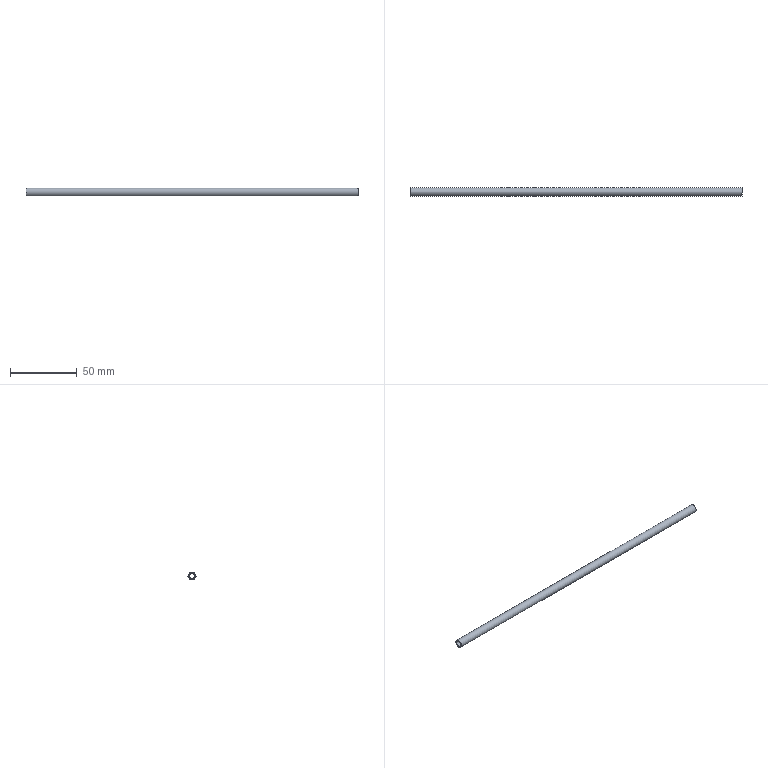Part | NX | features solid 2 | 1 solid | 4 faces | box 248.824 x 6 x 6 mm | volume 3909 mm3 | cylinder 2 | plane 2 | commonest cylinder face diameters 4 x1 6 x1
STEP:
#1=CARTESIAN_POINT('',(-323.824,-70.,347.));
#2=VERTEX_POINT('',#1);
#3=CARTESIAN_POINT('',(-323.824,-68.,347.));
#4=DIRECTION('',(-1.,0.,0.));
#5=DIRECTION('',(0.,-1.,0.));
#6=AXIS2_PLACEMENT_3D('',#3,#4,#5);
#7=CIRCLE('',#6,2.);
#8=EDGE_CURVE('',#2,#2,#7,.T.);
#9=ORIENTED_EDGE('',*,*,#8,.T.);
#10=EDGE_LOOP('',(#9));
#11=FACE_BOUND('',#10,.T.);
#12=CARTESIAN_POINT('',(-75.,-70.,347.));
#13=VERTEX_POINT('',#12);
#14=CARTESIAN_POINT('',(-75.,-68.,347.));
#15=DIRECTION('',(-1.,0.,0.));
#16=DIRECTION('',(0.,-1.,0.));
#17=AXIS2_PLACEMENT_3D('',#14,#15,#16);
#18=CIRCLE('',#17,2.);
#19=EDGE_CURVE('',#13,#13,#18,.T.);
#20=ORIENTED_EDGE('',*,*,#19,.F.);
#21=EDGE_LOOP('',(#20));
#22=FACE_BOUND('',#21,.T.);
#23=CARTESIAN_POINT('',(-273.824,-68.,347.));
#24=DIRECTION('',(1.,0.,0.));
#25=DIRECTION('',(0.,1.,0.));
#26=AXIS2_PLACEMENT_3D('',#23,#24,#25);
#27=CYLINDRICAL_SURFACE('',#26,2.);
#28=ADVANCED_FACE('',(#11,#22),#27,.F.);
#29=CARTESIAN_POINT('',(-323.824,-71.,347.));
#30=VERTEX_POINT('',#29);
#31=CARTESIAN_POINT('',(-323.824,-68.,347.));
#32=DIRECTION('',(-1.,0.,0.));
#33=DIRECTION('',(0.,-1.,0.));
#34=AXIS2_PLACEMENT_3D('',#31,#32,#33);
#35=CIRCLE('',#34,3.);
#36=EDGE_CURVE('',#30,#30,#35,.T.);
#37=ORIENTED_EDGE('',*,*,#36,.F.);
#38=EDGE_LOOP('',(#37));
#39=FACE_BOUND('',#38,.T.);
#40=CARTESIAN_POINT('',(-75.,-71.,347.));
#41=VERTEX_POINT('',#40);
#42=CARTESIAN_POINT('',(-75.,-68.,347.));
#43=DIRECTION('',(-1.,0.,0.));
#44=DIRECTION('',(0.,-1.,0.));
#45=AXIS2_PLACEMENT_3D('',#42,#43,#44);
#46=CIRCLE('',#45,3.);
#47=EDGE_CURVE('',#41,#41,#46,.T.);
#48=ORIENTED_EDGE('',*,*,#47,.T.);
#49=EDGE_LOOP('',(#48));
#50=FACE_BOUND('',#49,.T.);
#51=CARTESIAN_POINT('',(-273.824,-68.,347.));
#52=DIRECTION('',(1.,0.,0.));
#53=DIRECTION('',(0.,1.,0.));
#54=AXIS2_PLACEMENT_3D('',#51,#52,#53);
#55=CYLINDRICAL_SURFACE('',#54,3.);
#56=ADVANCED_FACE('',(#39,#50),#55,.T.);
#57=ORIENTED_EDGE('',*,*,#8,.F.);
#58=EDGE_LOOP('',(#57));
#59=FACE_BOUND('',#58,.T.);
#60=ORIENTED_EDGE('',*,*,#36,.T.);
#61=EDGE_LOOP('',(#60));
#62=FACE_BOUND('',#61,.T.);
#63=CARTESIAN_POINT('',(-323.824,-68.,347.));
#64=DIRECTION('',(-1.,0.,0.));
#65=DIRECTION('',(0.,-1.,0.));
#66=AXIS2_PLACEMENT_3D('',#63,#64,#65);
#67=PLANE('',#66);
#68=ADVANCED_FACE('',(#59,#62),#67,.T.);
#69=ORIENTED_EDGE('',*,*,#19,.T.);
#70=EDGE_LOOP('',(#69));
#71=FACE_BOUND('',#70,.T.);
#72=ORIENTED_EDGE('',*,*,#47,.F.);
#73=EDGE_LOOP('',(#72));
#74=FACE_BOUND('',#73,.T.);
#75=CARTESIAN_POINT('',(-75.,-68.,347.));
#76=DIRECTION('',(-1.,0.,0.));
#77=DIRECTION('',(0.,-1.,0.));
#78=AXIS2_PLACEMENT_3D('',#75,#76,#77);
#79=PLANE('',#78);
#80=ADVANCED_FACE('',(#71,#74),#79,.F.);
#81=CLOSED_SHELL('',(#28,#56,#68,#80));
#82=MANIFOLD_SOLID_BREP('',#81);
#83=(LENGTH_UNIT()NAMED_UNIT(*)SI_UNIT(.MILLI.,.METRE.));
#84=UNCERTAINTY_MEASURE_WITH_UNIT(LENGTH_MEASURE(0.00001),#83,'','');
#85=(NAMED_UNIT(*)PLANE_ANGLE_UNIT()SI_UNIT($,.RADIAN.));
#86=(NAMED_UNIT(*)SI_UNIT($,.STERADIAN.)SOLID_ANGLE_UNIT());
#87=(GEOMETRIC_REPRESENTATION_CONTEXT(3)GLOBAL_UNCERTAINTY_ASSIGNED_CONTEXT((#84))GLOBAL_UNIT_ASSIGNED_CONTEXT((#83,#85,#86))REPRESENTATION_CONTEXT('',''));
#88=ADVANCED_BREP_SHAPE_REPRESENTATION('',(#82),#87);